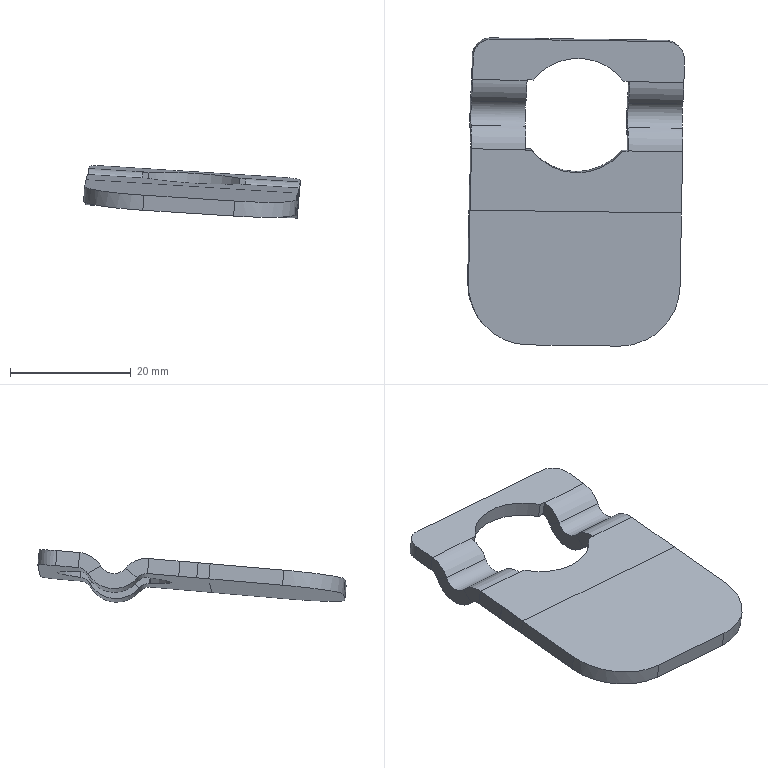Part | 1 solid | 55 faces | box 35.842 x 50.971 x 8.67 mm | volume 3721 mm3 | plane 24 | spline 16 | cylinder 14 | other 1 | commonest cylinder face diameters 4 x4 9 x4 6 x2 19 x2 20 x2